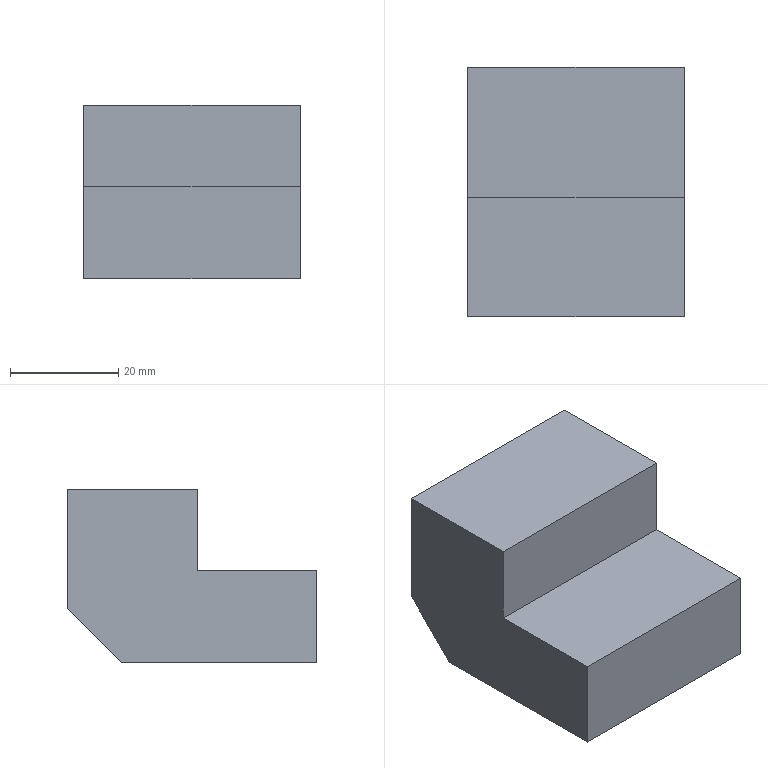Part | STEP file | ASND-0110-Body 1-29 | 1 solid | 9 faces | box 40 x 46 x 32 mm | volume 43680 mm3 | plane 9
STEP:
#1=CARTESIAN_POINT('',(0.,0.,0.));
#2=DIRECTION('',(0.,0.,1.));
#3=DIRECTION('',(1.,0.,0.));
#4=AXIS2_PLACEMENT_3D('',#1,#2,#3);
#5=CARTESIAN_POINT('',(0.,14.,-12.));
#6=VERTEX_POINT('',#5);
#7=CARTESIAN_POINT('',(0.,24.,-2.));
#8=VERTEX_POINT('',#7);
#9=CARTESIAN_POINT('',(0.,16.,-10.));
#10=DIRECTION('',(0.,0.7071,0.7071));
#11=VECTOR('',#10,1.);
#12=LINE('',#9,#11);
#13=CARTESIAN_POINT('',(13.5,19.,-7.));
#14=DIRECTION('',(0.,0.7071,-0.7071));
#15=DIRECTION('',(0.5774,0.5774,0.5774));
#16=AXIS2_PLACEMENT_3D('',#13,#14,#15);
#17=PLANE('',#16);
#18=CARTESIAN_POINT('',(-11.258,-8.573));
#19=DIRECTION('',(0.8165,-0.5774));
#20=VECTOR('',#19,1.);
#21=LINE('',#18,#20);
#22=(GEOMETRIC_REPRESENTATION_CONTEXT(2)PARAMETRIC_REPRESENTATION_CONTEXT()REPRESENTATION_CONTEXT('',''));
#23=DEFINITIONAL_REPRESENTATION('',(#21),#22);
#24=PCURVE('',#17,#23);
#25=CARTESIAN_POINT('',(0.,0.,0.));
#26=DIRECTION('',(-1.,0.,0.));
#27=DIRECTION('',(0.,0.7071,0.7071));
#28=AXIS2_PLACEMENT_3D('',#25,#26,#27);
#29=PLANE('',#28);
#30=CARTESIAN_POINT('',(4.243,18.385));
#31=DIRECTION('',(1.,0.));
#32=VECTOR('',#31,1.);
#33=LINE('',#30,#32);
#34=(GEOMETRIC_REPRESENTATION_CONTEXT(2)PARAMETRIC_REPRESENTATION_CONTEXT()REPRESENTATION_CONTEXT('',''));
#35=DEFINITIONAL_REPRESENTATION('',(#33),#34);
#36=PCURVE('',#29,#35);
#37=SURFACE_CURVE('',#12,(#24,#36),.PCURVE_S1.);
#38=EDGE_CURVE('',#6,#8,#37,.T.);
#39=ORIENTED_EDGE('',*,*,#38,.T.);
#40=CARTESIAN_POINT('',(40.,24.,-2.));
#41=VERTEX_POINT('',#40);
#42=CARTESIAN_POINT('',(13.5,24.,-2.));
#43=DIRECTION('',(1.,0.,0.));
#44=VECTOR('',#43,1.);
#45=LINE('',#42,#44);
#46=CARTESIAN_POINT('',(5.774,-4.082));
#47=DIRECTION('',(0.5774,0.8165));
#48=VECTOR('',#47,1.);
#49=LINE('',#46,#48);
#50=(GEOMETRIC_REPRESENTATION_CONTEXT(2)PARAMETRIC_REPRESENTATION_CONTEXT()REPRESENTATION_CONTEXT('',''));
#51=DEFINITIONAL_REPRESENTATION('',(#49),#50);
#52=PCURVE('',#17,#51);
#53=CARTESIAN_POINT('',(0.,24.,0.));
#54=DIRECTION('',(0.,1.,0.));
#55=DIRECTION('',(0.7071,0.,0.7071));
#56=AXIS2_PLACEMENT_3D('',#53,#54,#55);
#57=PLANE('',#56);
#58=CARTESIAN_POINT('',(8.132,10.96));
#59=DIRECTION('',(0.7071,0.7071));
#60=VECTOR('',#59,1.);
#61=LINE('',#58,#60);
#62=(GEOMETRIC_REPRESENTATION_CONTEXT(2)PARAMETRIC_REPRESENTATION_CONTEXT()REPRESENTATION_CONTEXT('',''));
#63=DEFINITIONAL_REPRESENTATION('',(#61),#62);
#64=PCURVE('',#57,#63);
#65=SURFACE_CURVE('',#45,(#52,#64),.PCURVE_S1.);
#66=EDGE_CURVE('',#8,#41,#65,.T.);
#67=ORIENTED_EDGE('',*,*,#66,.T.);
#68=CARTESIAN_POINT('',(40.,14.,-12.));
#69=VERTEX_POINT('',#68);
#70=CARTESIAN_POINT('',(40.,22.,-4.));
#71=DIRECTION('',(0.,-0.7071,-0.7071));
#72=VECTOR('',#71,1.);
#73=LINE('',#70,#72);
#74=CARTESIAN_POINT('',(18.764,19.188));
#75=DIRECTION('',(-0.8165,0.5774));
#76=VECTOR('',#75,1.);
#77=LINE('',#74,#76);
#78=(GEOMETRIC_REPRESENTATION_CONTEXT(2)PARAMETRIC_REPRESENTATION_CONTEXT()REPRESENTATION_CONTEXT('',''));
#79=DEFINITIONAL_REPRESENTATION('',(#77),#78);
#80=PCURVE('',#17,#79);
#81=CARTESIAN_POINT('',(40.,24.,0.));
#82=DIRECTION('',(1.,0.,0.));
#83=DIRECTION('',(0.,0.7071,0.7071));
#84=AXIS2_PLACEMENT_3D('',#81,#82,#83);
#85=PLANE('',#84);
#86=CARTESIAN_POINT('',(-4.243,-1.414));
#87=DIRECTION('',(-1.,0.));
#88=VECTOR('',#87,1.);
#89=LINE('',#86,#88);
#90=(GEOMETRIC_REPRESENTATION_CONTEXT(2)PARAMETRIC_REPRESENTATION_CONTEXT()REPRESENTATION_CONTEXT('',''));
#91=DEFINITIONAL_REPRESENTATION('',(#89),#90);
#92=PCURVE('',#85,#91);
#93=SURFACE_CURVE('',#73,(#80,#92),.PCURVE_S1.);
#94=EDGE_CURVE('',#41,#69,#93,.T.);
#95=ORIENTED_EDGE('',*,*,#94,.T.);
#96=CARTESIAN_POINT('',(13.5,14.,-12.));
#97=DIRECTION('',(-1.,0.,0.));
#98=VECTOR('',#97,1.);
#99=LINE('',#96,#98);
#100=CARTESIAN_POINT('',(-5.774,4.082));
#101=DIRECTION('',(-0.5774,-0.8165));
#102=VECTOR('',#101,1.);
#103=LINE('',#100,#102);
#104=(GEOMETRIC_REPRESENTATION_CONTEXT(2)PARAMETRIC_REPRESENTATION_CONTEXT()REPRESENTATION_CONTEXT('',''));
#105=DEFINITIONAL_REPRESENTATION('',(#103),#104);
#106=PCURVE('',#17,#105);
#107=CARTESIAN_POINT('',(27.,12.,-12.));
#108=DIRECTION('',(0.,0.,1.));
#109=DIRECTION('',(0.7071,0.7071,0.));
#110=AXIS2_PLACEMENT_3D('',#107,#108,#109);
#111=PLANE('',#110);
#112=CARTESIAN_POINT('',(-8.132,10.96));
#113=DIRECTION('',(-0.7071,0.7071));
#114=VECTOR('',#113,1.);
#115=LINE('',#112,#114);
#116=(GEOMETRIC_REPRESENTATION_CONTEXT(2)PARAMETRIC_REPRESENTATION_CONTEXT()REPRESENTATION_CONTEXT('',''));
#117=DEFINITIONAL_REPRESENTATION('',(#115),#116);
#118=PCURVE('',#111,#117);
#119=SURFACE_CURVE('',#99,(#106,#118),.PCURVE_S1.);
#120=EDGE_CURVE('',#69,#6,#119,.T.);
#121=ORIENTED_EDGE('',*,*,#120,.T.);
#122=EDGE_LOOP('',(#39,#67,#95,#121));
#123=FACE_BOUND('',#122,.T.);
#124=ADVANCED_FACE('',(#123),#17,.T.);
#125=ORIENTED_EDGE('',*,*,#66,.F.);
#126=CARTESIAN_POINT('',(0.,24.,20.));
#127=VERTEX_POINT('',#126);
#128=CARTESIAN_POINT('',(0.,24.,0.));
#129=DIRECTION('',(0.,0.,1.));
#130=VECTOR('',#129,1.);
#131=LINE('',#128,#130);
#132=CARTESIAN_POINT('',(0.,0.));
#133=DIRECTION('',(0.7071,-0.7071));
#134=VECTOR('',#133,1.);
#135=LINE('',#132,#134);
#136=(GEOMETRIC_REPRESENTATION_CONTEXT(2)PARAMETRIC_REPRESENTATION_CONTEXT()REPRESENTATION_CONTEXT('',''));
#137=DEFINITIONAL_REPRESENTATION('',(#135),#136);
#138=PCURVE('',#57,#137);
#139=CARTESIAN_POINT('',(16.971,16.971));
#140=DIRECTION('',(0.7071,-0.7071));
#141=VECTOR('',#140,1.);
#142=LINE('',#139,#141);
#143=(GEOMETRIC_REPRESENTATION_CONTEXT(2)PARAMETRIC_REPRESENTATION_CONTEXT()REPRESENTATION_CONTEXT('',''));
#144=DEFINITIONAL_REPRESENTATION('',(#142),#143);
#145=PCURVE('',#29,#144);
#146=SURFACE_CURVE('',#131,(#138,#145),.PCURVE_S1.);
#147=EDGE_CURVE('',#8,#127,#146,.T.);
#148=ORIENTED_EDGE('',*,*,#147,.T.);
#149=CARTESIAN_POINT('',(40.,24.,20.));
#150=VERTEX_POINT('',#149);
#151=CARTESIAN_POINT('',(54.,24.,20.));
#152=DIRECTION('',(1.,0.,0.));
#153=VECTOR('',#152,1.);
#154=LINE('',#151,#153);
#155=CARTESIAN_POINT('',(52.326,24.042));
#156=DIRECTION('',(0.7071,0.7071));
#157=VECTOR('',#156,1.);
#158=LINE('',#155,#157);
#159=(GEOMETRIC_REPRESENTATION_CONTEXT(2)PARAMETRIC_REPRESENTATION_CONTEXT()REPRESENTATION_CONTEXT('',''));
#160=DEFINITIONAL_REPRESENTATION('',(#158),#159);
#161=PCURVE('',#57,#160);
#162=CARTESIAN_POINT('',(27.,12.,20.));
#163=DIRECTION('',(0.,0.,1.));
#164=DIRECTION('',(0.7071,0.7071,0.));
#165=AXIS2_PLACEMENT_3D('',#162,#163,#164);
#166=PLANE('',#165);
#167=CARTESIAN_POINT('',(27.577,-10.607));
#168=DIRECTION('',(0.7071,-0.7071));
#169=VECTOR('',#168,1.);
#170=LINE('',#167,#169);
#171=(GEOMETRIC_REPRESENTATION_CONTEXT(2)PARAMETRIC_REPRESENTATION_CONTEXT()REPRESENTATION_CONTEXT('',''));
#172=DEFINITIONAL_REPRESENTATION('',(#170),#171);
#173=PCURVE('',#166,#172);
#174=SURFACE_CURVE('',#154,(#161,#173),.PCURVE_S1.);
#175=EDGE_CURVE('',#127,#150,#174,.T.);
#176=ORIENTED_EDGE('',*,*,#175,.T.);
#177=CARTESIAN_POINT('',(40.,24.,0.));
#178=DIRECTION('',(0.,0.,1.));
#179=VECTOR('',#178,1.);
#180=LINE('',#177,#179);
#181=CARTESIAN_POINT('',(28.284,28.284));
#182=DIRECTION('',(0.7071,-0.7071));
#183=VECTOR('',#182,1.);
#184=LINE('',#181,#183);
#185=(GEOMETRIC_REPRESENTATION_CONTEXT(2)PARAMETRIC_REPRESENTATION_CONTEXT()REPRESENTATION_CONTEXT('',''));
#186=DEFINITIONAL_REPRESENTATION('',(#184),#185);
#187=PCURVE('',#57,#186);
#188=CARTESIAN_POINT('',(0.,0.));
#189=DIRECTION('',(0.7071,0.7071));
#190=VECTOR('',#189,1.);
#191=LINE('',#188,#190);
#192=(GEOMETRIC_REPRESENTATION_CONTEXT(2)PARAMETRIC_REPRESENTATION_CONTEXT()REPRESENTATION_CONTEXT('',''));
#193=DEFINITIONAL_REPRESENTATION('',(#191),#192);
#194=PCURVE('',#85,#193);
#195=SURFACE_CURVE('',#180,(#187,#194),.PCURVE_S1.);
#196=EDGE_CURVE('',#41,#150,#195,.T.);
#197=ORIENTED_EDGE('',*,*,#196,.F.);
#198=EDGE_LOOP('',(#125,#148,#176,#197));
#199=FACE_BOUND('',#198,.T.);
#200=ADVANCED_FACE('',(#199),#57,.T.);
#201=ORIENTED_EDGE('',*,*,#38,.F.);
#202=CARTESIAN_POINT('',(0.,-22.,-12.));
#203=VERTEX_POINT('',#202);
#204=CARTESIAN_POINT('',(0.,24.,-12.));
#205=DIRECTION('',(0.,-1.,0.));
#206=VECTOR('',#205,1.);
#207=LINE('',#204,#206);
#208=CARTESIAN_POINT('',(8.485,25.456));
#209=DIRECTION('',(-0.7071,-0.7071));
#210=VECTOR('',#209,1.);
#211=LINE('',#208,#210);
#212=(GEOMETRIC_REPRESENTATION_CONTEXT(2)PARAMETRIC_REPRESENTATION_CONTEXT()REPRESENTATION_CONTEXT('',''));
#213=DEFINITIONAL_REPRESENTATION('',(#211),#212);
#214=PCURVE('',#29,#213);
#215=CARTESIAN_POINT('',(-10.607,27.577));
#216=DIRECTION('',(-0.7071,-0.7071));
#217=VECTOR('',#216,1.);
#218=LINE('',#215,#217);
#219=(GEOMETRIC_REPRESENTATION_CONTEXT(2)PARAMETRIC_REPRESENTATION_CONTEXT()REPRESENTATION_CONTEXT('',''));
#220=DEFINITIONAL_REPRESENTATION('',(#218),#219);
#221=PCURVE('',#111,#220);
#222=SURFACE_CURVE('',#207,(#214,#221),.PCURVE_S1.);
#223=EDGE_CURVE('',#6,#203,#222,.T.);
#224=ORIENTED_EDGE('',*,*,#223,.T.);
#225=CARTESIAN_POINT('',(0.,-22.,5.));
#226=VERTEX_POINT('',#225);
#227=CARTESIAN_POINT('',(0.,-22.,0.));
#228=DIRECTION('',(0.,0.,1.));
#229=VECTOR('',#228,1.);
#230=LINE('',#227,#229);
#231=CARTESIAN_POINT('',(-15.556,-15.556));
#232=DIRECTION('',(0.7071,-0.7071));
#233=VECTOR('',#232,1.);
#234=LINE('',#231,#233);
#235=(GEOMETRIC_REPRESENTATION_CONTEXT(2)PARAMETRIC_REPRESENTATION_CONTEXT()REPRESENTATION_CONTEXT('',''));
#236=DEFINITIONAL_REPRESENTATION('',(#234),#235);
#237=PCURVE('',#29,#236);
#238=CARTESIAN_POINT('',(27.,-22.,-6.));
#239=DIRECTION('',(0.,1.,0.));
#240=DIRECTION('',(0.7071,0.,0.7071));
#241=AXIS2_PLACEMENT_3D('',#238,#239,#240);
#242=PLANE('',#241);
#243=CARTESIAN_POINT('',(-14.849,-23.335));
#244=DIRECTION('',(0.7071,-0.7071));
#245=VECTOR('',#244,1.);
#246=LINE('',#243,#245);
#247=(GEOMETRIC_REPRESENTATION_CONTEXT(2)PARAMETRIC_REPRESENTATION_CONTEXT()REPRESENTATION_CONTEXT('',''));
#248=DEFINITIONAL_REPRESENTATION('',(#246),#247);
#249=PCURVE('',#242,#248);
#250=SURFACE_CURVE('',#230,(#237,#249),.PCURVE_S1.);
#251=EDGE_CURVE('',#203,#226,#250,.T.);
#252=ORIENTED_EDGE('',*,*,#251,.T.);
#253=CARTESIAN_POINT('',(0.,0.,5.));
#254=VERTEX_POINT('',#253);
#255=CARTESIAN_POINT('',(0.,0.,5.));
#256=DIRECTION('',(0.,-1.,0.));
#257=VECTOR('',#256,1.);
#258=LINE('',#255,#257);
#259=CARTESIAN_POINT('',(3.536,-3.536));
#260=DIRECTION('',(-0.7071,-0.7071));
#261=VECTOR('',#260,1.);
#262=LINE('',#259,#261);
#263=(GEOMETRIC_REPRESENTATION_CONTEXT(2)PARAMETRIC_REPRESENTATION_CONTEXT()REPRESENTATION_CONTEXT('',''));
#264=DEFINITIONAL_REPRESENTATION('',(#262),#263);
#265=PCURVE('',#29,#264);
#266=CARTESIAN_POINT('',(0.,0.,5.));
#267=DIRECTION('',(0.,0.,1.));
#268=DIRECTION('',(0.7071,0.7071,0.));
#269=AXIS2_PLACEMENT_3D('',#266,#267,#268);
#270=PLANE('',#269);
#271=CARTESIAN_POINT('',(0.,0.));
#272=DIRECTION('',(-0.7071,-0.7071));
#273=VECTOR('',#272,1.);
#274=LINE('',#271,#273);
#275=(GEOMETRIC_REPRESENTATION_CONTEXT(2)PARAMETRIC_REPRESENTATION_CONTEXT()REPRESENTATION_CONTEXT('',''));
#276=DEFINITIONAL_REPRESENTATION('',(#274),#275);
#277=PCURVE('',#270,#276);
#278=SURFACE_CURVE('',#258,(#265,#277),.PCURVE_S1.);
#279=EDGE_CURVE('',#254,#226,#278,.T.);
#280=ORIENTED_EDGE('',*,*,#279,.F.);
#281=CARTESIAN_POINT('',(0.,0.,20.));
#282=VERTEX_POINT('',#281);
#283=CARTESIAN_POINT('',(0.,0.,0.));
#284=DIRECTION('',(0.,0.,1.));
#285=VECTOR('',#284,1.);
#286=LINE('',#283,#285);
#287=CARTESIAN_POINT('',(0.,0.));
#288=DIRECTION('',(0.7071,-0.7071));
#289=VECTOR('',#288,1.);
#290=LINE('',#287,#289);
#291=(GEOMETRIC_REPRESENTATION_CONTEXT(2)PARAMETRIC_REPRESENTATION_CONTEXT()REPRESENTATION_CONTEXT('',''));
#292=DEFINITIONAL_REPRESENTATION('',(#290),#291);
#293=PCURVE('',#29,#292);
#294=CARTESIAN_POINT('',(54.,0.,0.));
#295=DIRECTION('',(0.,-1.,0.));
#296=DIRECTION('',(0.7071,0.,0.7071));
#297=AXIS2_PLACEMENT_3D('',#294,#295,#296);
#298=PLANE('',#297);
#299=CARTESIAN_POINT('',(-38.184,38.184));
#300=DIRECTION('',(0.7071,0.7071));
#301=VECTOR('',#300,1.);
#302=LINE('',#299,#301);
#303=(GEOMETRIC_REPRESENTATION_CONTEXT(2)PARAMETRIC_REPRESENTATION_CONTEXT()REPRESENTATION_CONTEXT('',''));
#304=DEFINITIONAL_REPRESENTATION('',(#302),#303);
#305=PCURVE('',#298,#304);
#306=SURFACE_CURVE('',#286,(#293,#305),.PCURVE_S1.);
#307=EDGE_CURVE('',#254,#282,#306,.T.);
#308=ORIENTED_EDGE('',*,*,#307,.T.);
#309=CARTESIAN_POINT('',(0.,24.,20.));
#310=DIRECTION('',(0.,1.,0.));
#311=VECTOR('',#310,1.);
#312=LINE('',#309,#311);
#313=CARTESIAN_POINT('',(31.113,2.828));
#314=DIRECTION('',(0.7071,0.7071));
#315=VECTOR('',#314,1.);
#316=LINE('',#313,#315);
#317=(GEOMETRIC_REPRESENTATION_CONTEXT(2)PARAMETRIC_REPRESENTATION_CONTEXT()REPRESENTATION_CONTEXT('',''));
#318=DEFINITIONAL_REPRESENTATION('',(#316),#317);
#319=PCURVE('',#29,#318);
#320=CARTESIAN_POINT('',(-10.607,27.577));
#321=DIRECTION('',(0.7071,0.7071));
#322=VECTOR('',#321,1.);
#323=LINE('',#320,#322);
#324=(GEOMETRIC_REPRESENTATION_CONTEXT(2)PARAMETRIC_REPRESENTATION_CONTEXT()REPRESENTATION_CONTEXT('',''));
#325=DEFINITIONAL_REPRESENTATION('',(#323),#324);
#326=PCURVE('',#166,#325);
#327=SURFACE_CURVE('',#312,(#319,#326),.PCURVE_S1.);
#328=EDGE_CURVE('',#282,#127,#327,.T.);
#329=ORIENTED_EDGE('',*,*,#328,.T.);
#330=ORIENTED_EDGE('',*,*,#147,.F.);
#331=EDGE_LOOP('',(#201,#224,#252,#280,#308,#329,#330));
#332=FACE_BOUND('',#331,.T.);
#333=ADVANCED_FACE('',(#332),#29,.T.);
#334=CARTESIAN_POINT('',(40.,-22.,5.));
#335=VERTEX_POINT('',#334);
#336=CARTESIAN_POINT('',(54.,-22.,5.));
#337=DIRECTION('',(1.,0.,0.));
#338=VECTOR('',#337,1.);
#339=LINE('',#336,#338);
#340=CARTESIAN_POINT('',(22.627,-53.74));
#341=DIRECTION('',(0.7071,-0.7071));
#342=VECTOR('',#341,1.);
#343=LINE('',#340,#342);
#344=(GEOMETRIC_REPRESENTATION_CONTEXT(2)PARAMETRIC_REPRESENTATION_CONTEXT()REPRESENTATION_CONTEXT('',''));
#345=DEFINITIONAL_REPRESENTATION('',(#343),#344);
#346=PCURVE('',#270,#345);
#347=CARTESIAN_POINT('',(26.87,11.314));
#348=DIRECTION('',(0.7071,0.7071));
#349=VECTOR('',#348,1.);
#350=LINE('',#347,#349);
#351=(GEOMETRIC_REPRESENTATION_CONTEXT(2)PARAMETRIC_REPRESENTATION_CONTEXT()REPRESENTATION_CONTEXT('',''));
#352=DEFINITIONAL_REPRESENTATION('',(#350),#351);
#353=PCURVE('',#242,#352);
#354=SURFACE_CURVE('',#339,(#346,#353),.PCURVE_S1.);
#355=EDGE_CURVE('',#226,#335,#354,.T.);
#356=ORIENTED_EDGE('',*,*,#355,.T.);
#357=CARTESIAN_POINT('',(40.,0.,5.));
#358=VERTEX_POINT('',#357);
#359=CARTESIAN_POINT('',(40.,0.,5.));
#360=DIRECTION('',(0.,-1.,0.));
#361=VECTOR('',#360,1.);
#362=LINE('',#359,#361);
#363=CARTESIAN_POINT('',(28.284,-28.284));
#364=DIRECTION('',(-0.7071,-0.7071));
#365=VECTOR('',#364,1.);
#366=LINE('',#363,#365);
#367=(GEOMETRIC_REPRESENTATION_CONTEXT(2)PARAMETRIC_REPRESENTATION_CONTEXT()REPRESENTATION_CONTEXT('',''));
#368=DEFINITIONAL_REPRESENTATION('',(#366),#367);
#369=PCURVE('',#270,#368);
#370=CARTESIAN_POINT('',(-13.435,20.506));
#371=DIRECTION('',(-0.7071,0.7071));
#372=VECTOR('',#371,1.);
#373=LINE('',#370,#372);
#374=(GEOMETRIC_REPRESENTATION_CONTEXT(2)PARAMETRIC_REPRESENTATION_CONTEXT()REPRESENTATION_CONTEXT('',''));
#375=DEFINITIONAL_REPRESENTATION('',(#373),#374);
#376=PCURVE('',#85,#375);
#377=SURFACE_CURVE('',#362,(#369,#376),.PCURVE_S1.);
#378=EDGE_CURVE('',#358,#335,#377,.T.);
#379=ORIENTED_EDGE('',*,*,#378,.F.);
#380=CARTESIAN_POINT('',(27.,0.,5.));
#381=DIRECTION('',(1.,0.,0.));
#382=VECTOR('',#381,1.);
#383=LINE('',#380,#382);
#384=CARTESIAN_POINT('',(19.092,-19.092));
#385=DIRECTION('',(0.7071,-0.7071));
#386=VECTOR('',#385,1.);
#387=LINE('',#384,#386);
#388=(GEOMETRIC_REPRESENTATION_CONTEXT(2)PARAMETRIC_REPRESENTATION_CONTEXT()REPRESENTATION_CONTEXT('',''));
#389=DEFINITIONAL_REPRESENTATION('',(#387),#388);
#390=PCURVE('',#270,#389);
#391=CARTESIAN_POINT('',(-15.556,22.627));
#392=DIRECTION('',(0.7071,-0.7071));
#393=VECTOR('',#392,1.);
#394=LINE('',#391,#393);
#395=(GEOMETRIC_REPRESENTATION_CONTEXT(2)PARAMETRIC_REPRESENTATION_CONTEXT()REPRESENTATION_CONTEXT('',''));
#396=DEFINITIONAL_REPRESENTATION('',(#394),#395);
#397=PCURVE('',#298,#396);
#398=SURFACE_CURVE('',#383,(#390,#397),.PCURVE_S1.);
#399=EDGE_CURVE('',#254,#358,#398,.T.);
#400=ORIENTED_EDGE('',*,*,#399,.F.);
#401=ORIENTED_EDGE('',*,*,#279,.T.);
#402=EDGE_LOOP('',(#356,#379,#400,#401));
#403=FACE_BOUND('',#402,.T.);
#404=ADVANCED_FACE('',(#403),#270,.T.);
#405=ORIENTED_EDGE('',*,*,#251,.F.);
#406=CARTESIAN_POINT('',(40.,-22.,-12.));
#407=VERTEX_POINT('',#406);
#408=CARTESIAN_POINT('',(0.,-22.,-12.));
#409=DIRECTION('',(-1.,0.,0.));
#410=VECTOR('',#409,1.);
#411=LINE('',#408,#410);
#412=CARTESIAN_POINT('',(-23.335,-14.849));
#413=DIRECTION('',(-0.7071,-0.7071));
#414=VECTOR('',#413,1.);
#415=LINE('',#412,#414);
#416=(GEOMETRIC_REPRESENTATION_CONTEXT(2)PARAMETRIC_REPRESENTATION_CONTEXT()REPRESENTATION_CONTEXT('',''));
#417=DEFINITIONAL_REPRESENTATION('',(#415),#416);
#418=PCURVE('',#242,#417);
#419=CARTESIAN_POINT('',(-43.134,-4.95));
#420=DIRECTION('',(-0.7071,0.7071));
#421=VECTOR('',#420,1.);
#422=LINE('',#419,#421);
#423=(GEOMETRIC_REPRESENTATION_CONTEXT(2)PARAMETRIC_REPRESENTATION_CONTEXT()REPRESENTATION_CONTEXT('',''));
#424=DEFINITIONAL_REPRESENTATION('',(#422),#423);
#425=PCURVE('',#111,#424);
#426=SURFACE_CURVE('',#411,(#418,#425),.PCURVE_S1.);
#427=EDGE_CURVE('',#407,#203,#426,.T.);
#428=ORIENTED_EDGE('',*,*,#427,.F.);
#429=CARTESIAN_POINT('',(40.,-22.,-12.));
#430=DIRECTION('',(0.,0.,-1.));
#431=VECTOR('',#430,1.);
#432=LINE('',#429,#431);
#433=CARTESIAN_POINT('',(4.95,13.435));
#434=DIRECTION('',(-0.7071,0.7071));
#435=VECTOR('',#434,1.);
#436=LINE('',#433,#435);
#437=(GEOMETRIC_REPRESENTATION_CONTEXT(2)PARAMETRIC_REPRESENTATION_CONTEXT()REPRESENTATION_CONTEXT('',''));
#438=DEFINITIONAL_REPRESENTATION('',(#436),#437);
#439=PCURVE('',#242,#438);
#440=CARTESIAN_POINT('',(-41.012,24.042));
#441=DIRECTION('',(-0.7071,-0.7071));
#442=VECTOR('',#441,1.);
#443=LINE('',#440,#442);
#444=(GEOMETRIC_REPRESENTATION_CONTEXT(2)PARAMETRIC_REPRESENTATION_CONTEXT()REPRESENTATION_CONTEXT('',''));
#445=DEFINITIONAL_REPRESENTATION('',(#443),#444);
#446=PCURVE('',#85,#445);
#447=SURFACE_CURVE('',#432,(#439,#446),.PCURVE_S1.);
#448=EDGE_CURVE('',#335,#407,#447,.T.);
#449=ORIENTED_EDGE('',*,*,#448,.F.);
#450=ORIENTED_EDGE('',*,*,#355,.F.);
#451=EDGE_LOOP('',(#405,#428,#449,#450));
#452=FACE_BOUND('',#451,.T.);
#453=ADVANCED_FACE('',(#452),#242,.F.);
#454=ORIENTED_EDGE('',*,*,#94,.F.);
#455=ORIENTED_EDGE('',*,*,#196,.T.);
#456=CARTESIAN_POINT('',(40.,0.,20.));
#457=VERTEX_POINT('',#456);
#458=CARTESIAN_POINT('',(40.,0.,20.));
#459=DIRECTION('',(0.,-1.,0.));
#460=VECTOR('',#459,1.);
#461=LINE('',#458,#460);
#462=CARTESIAN_POINT('',(-2.828,31.113));
#463=DIRECTION('',(-0.7071,0.7071));
#464=VECTOR('',#463,1.);
#465=LINE('',#462,#464);
#466=(GEOMETRIC_REPRESENTATION_CONTEXT(2)PARAMETRIC_REPRESENTATION_CONTEXT()REPRESENTATION_CONTEXT('',''));
#467=DEFINITIONAL_REPRESENTATION('',(#465),#466);
#468=PCURVE('',#85,#467);
#469=CARTESIAN_POINT('',(0.7071,-17.678));
#470=DIRECTION('',(-0.7071,-0.7071));
#471=VECTOR('',#470,1.);
#472=LINE('',#469,#471);
#473=(GEOMETRIC_REPRESENTATION_CONTEXT(2)PARAMETRIC_REPRESENTATION_CONTEXT()REPRESENTATION_CONTEXT('',''));
#474=DEFINITIONAL_REPRESENTATION('',(#472),#473);
#475=PCURVE('',#166,#474);
#476=SURFACE_CURVE('',#461,(#468,#475),.PCURVE_S1.);
#477=EDGE_CURVE('',#150,#457,#476,.T.);
#478=ORIENTED_EDGE('',*,*,#477,.T.);
#479=CARTESIAN_POINT('',(40.,0.,0.));
#480=DIRECTION('',(0.,0.,1.));
#481=VECTOR('',#480,1.);
#482=LINE('',#479,#481);
#483=CARTESIAN_POINT('',(-16.971,16.971));
#484=DIRECTION('',(0.7071,0.7071));
#485=VECTOR('',#484,1.);
#486=LINE('',#483,#485);
#487=(GEOMETRIC_REPRESENTATION_CONTEXT(2)PARAMETRIC_REPRESENTATION_CONTEXT()REPRESENTATION_CONTEXT('',''));
#488=DEFINITIONAL_REPRESENTATION('',(#486),#487);
#489=PCURVE('',#85,#488);
#490=CARTESIAN_POINT('',(-9.899,9.899));
#491=DIRECTION('',(0.7071,0.7071));
#492=VECTOR('',#491,1.);
#493=LINE('',#490,#492);
#494=(GEOMETRIC_REPRESENTATION_CONTEXT(2)PARAMETRIC_REPRESENTATION_CONTEXT()REPRESENTATION_CONTEXT('',''));
#495=DEFINITIONAL_REPRESENTATION('',(#493),#494);
#496=PCURVE('',#298,#495);
#497=SURFACE_CURVE('',#482,(#489,#496),.PCURVE_S1.);
#498=EDGE_CURVE('',#358,#457,#497,.T.);
#499=ORIENTED_EDGE('',*,*,#498,.F.);
#500=ORIENTED_EDGE('',*,*,#378,.T.);
#501=ORIENTED_EDGE('',*,*,#448,.T.);
#502=CARTESIAN_POINT('',(40.,0.,-12.));
#503=DIRECTION('',(0.,-1.,0.));
#504=VECTOR('',#503,1.);
#505=LINE('',#502,#504);
#506=CARTESIAN_POINT('',(-25.456,8.485));
#507=DIRECTION('',(-0.7071,0.7071));
#508=VECTOR('',#507,1.);
#509=LINE('',#506,#508);
#510=(GEOMETRIC_REPRESENTATION_CONTEXT(2)PARAMETRIC_REPRESENTATION_CONTEXT()REPRESENTATION_CONTEXT('',''));
#511=DEFINITIONAL_REPRESENTATION('',(#509),#510);
#512=PCURVE('',#85,#511);
#513=CARTESIAN_POINT('',(0.7071,-17.678));
#514=DIRECTION('',(-0.7071,-0.7071));
#515=VECTOR('',#514,1.);
#516=LINE('',#513,#515);
#517=(GEOMETRIC_REPRESENTATION_CONTEXT(2)PARAMETRIC_REPRESENTATION_CONTEXT()REPRESENTATION_CONTEXT('',''));
#518=DEFINITIONAL_REPRESENTATION('',(#516),#517);
#519=PCURVE('',#111,#518);
#520=SURFACE_CURVE('',#505,(#512,#519),.PCURVE_S1.);
#521=EDGE_CURVE('',#69,#407,#520,.T.);
#522=ORIENTED_EDGE('',*,*,#521,.F.);
#523=EDGE_LOOP('',(#454,#455,#478,#499,#500,#501,#522));
#524=FACE_BOUND('',#523,.T.);
#525=ADVANCED_FACE('',(#524),#85,.T.);
#526=ORIENTED_EDGE('',*,*,#399,.T.);
#527=ORIENTED_EDGE('',*,*,#498,.T.);
#528=CARTESIAN_POINT('',(0.,0.,20.));
#529=DIRECTION('',(-1.,0.,0.));
#530=VECTOR('',#529,1.);
#531=LINE('',#528,#530);
#532=CARTESIAN_POINT('',(-24.042,52.326));
#533=DIRECTION('',(-0.7071,0.7071));
#534=VECTOR('',#533,1.);
#535=LINE('',#532,#534);
#536=(GEOMETRIC_REPRESENTATION_CONTEXT(2)PARAMETRIC_REPRESENTATION_CONTEXT()REPRESENTATION_CONTEXT('',''));
#537=DEFINITIONAL_REPRESENTATION('',(#535),#536);
#538=PCURVE('',#298,#537);
#539=CARTESIAN_POINT('',(-27.577,10.607));
#540=DIRECTION('',(-0.7071,0.7071));
#541=VECTOR('',#540,1.);
#542=LINE('',#539,#541);
#543=(GEOMETRIC_REPRESENTATION_CONTEXT(2)PARAMETRIC_REPRESENTATION_CONTEXT()REPRESENTATION_CONTEXT('',''));
#544=DEFINITIONAL_REPRESENTATION('',(#542),#543);
#545=PCURVE('',#166,#544);
#546=SURFACE_CURVE('',#531,(#538,#545),.PCURVE_S1.);
#547=EDGE_CURVE('',#457,#282,#546,.T.);
#548=ORIENTED_EDGE('',*,*,#547,.T.);
#549=ORIENTED_EDGE('',*,*,#307,.F.);
#550=EDGE_LOOP('',(#526,#527,#548,#549));
#551=FACE_BOUND('',#550,.T.);
#552=ADVANCED_FACE('',(#551),#298,.T.);
#553=ORIENTED_EDGE('',*,*,#120,.F.);
#554=ORIENTED_EDGE('',*,*,#521,.T.);
#555=ORIENTED_EDGE('',*,*,#427,.T.);
#556=ORIENTED_EDGE('',*,*,#223,.F.);
#557=EDGE_LOOP('',(#553,#554,#555,#556));
#558=FACE_BOUND('',#557,.T.);
#559=ADVANCED_FACE('',(#558),#111,.F.);
#560=ORIENTED_EDGE('',*,*,#328,.F.);
#561=ORIENTED_EDGE('',*,*,#547,.F.);
#562=ORIENTED_EDGE('',*,*,#477,.F.);
#563=ORIENTED_EDGE('',*,*,#175,.F.);
#564=EDGE_LOOP('',(#560,#561,#562,#563));
#565=FACE_BOUND('',#564,.T.);
#566=ADVANCED_FACE('',(#565),#166,.T.);
#567=CLOSED_SHELL('',(#124,#200,#333,#404,#453,#525,#552,#559,#566));
#568=MANIFOLD_SOLID_BREP('',#567);
#569=(LENGTH_UNIT()NAMED_UNIT(*)SI_UNIT(.MILLI.,.METRE.));
#570=UNCERTAINTY_MEASURE_WITH_UNIT(LENGTH_MEASURE(0.0000001),#569,'','');
#571=(NAMED_UNIT(*)PLANE_ANGLE_UNIT()SI_UNIT($,.RADIAN.));
#572=(NAMED_UNIT(*)SI_UNIT($,.STERADIAN.)SOLID_ANGLE_UNIT());
#573=(GEOMETRIC_REPRESENTATION_CONTEXT(3)GLOBAL_UNCERTAINTY_ASSIGNED_CONTEXT((#570))GLOBAL_UNIT_ASSIGNED_CONTEXT((#569,#571,#572))REPRESENTATION_CONTEXT('',''));
#574=ADVANCED_BREP_SHAPE_REPRESENTATION('',(#4,#568),#573);